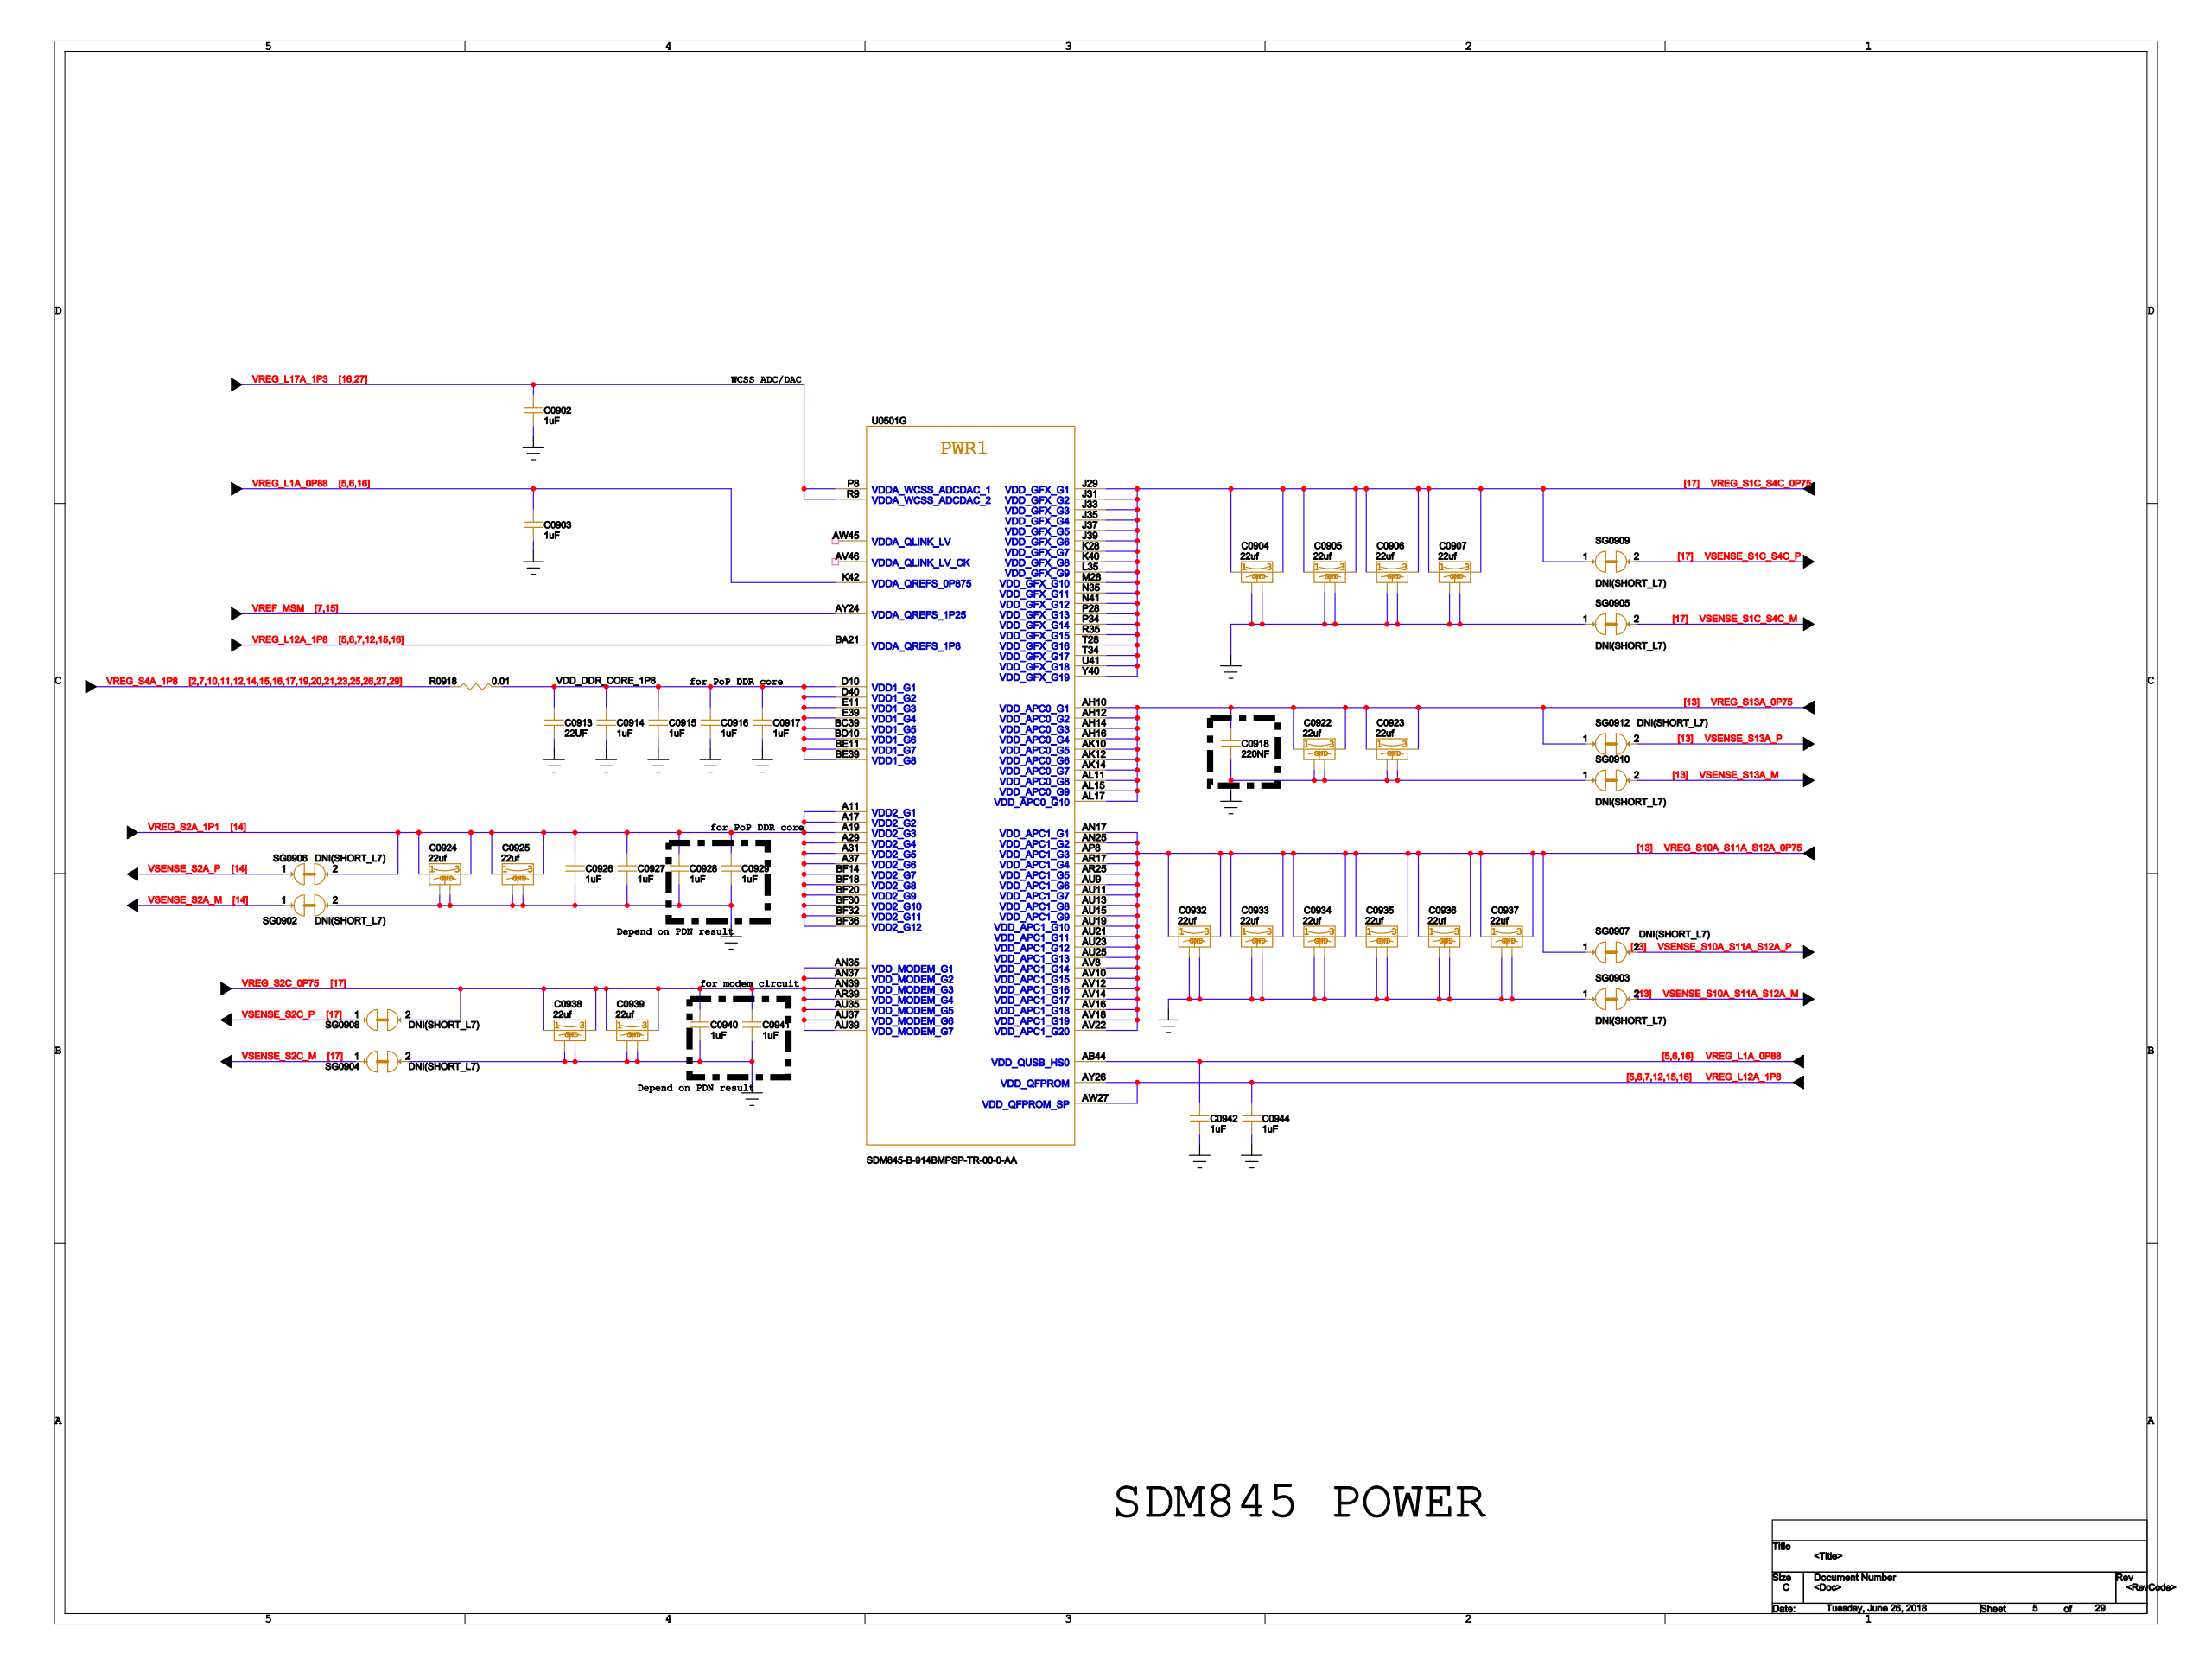Circuit board | Cadence Allegro | 802 parts | 566 nets | one sheet of the schematic
Parts on this sheet (reference | value | footprint):
C0902 | 1uF | C0201
C0903 | 1uF | C0201
C0904 | 22uf | NFMJMPC226R0G3
C0905 | 22uf | NFMJMPC226R0G3
C0906 | 22uf | NFMJMPC226R0G3
C0907 | 22uf | NFMJMPC226R0G3
C0913 | 22UF | 0603-BIG
C0914 | 1uF | C0201
C0915 | 1uF | C0201
C0916 | 1uF | C0201
C0917 | 1uF | C0201
C0918 | 220NF | C0201
C0922 | 22uf | NFMJMPC226R0G3
C0923 | 22uf | NFMJMPC226R0G3
C0924 | 22uf | NFMJMPC226R0G3
C0925 | 22uf | NFMJMPC226R0G3
C0926 | 1uF | C0201
C0927 | 1uF | C0201
C0928 | 1uF | C0201
C0929 | 1uF | C0201
C0932 | 22uf | NFMJMPC226R0G3
C0933 | 22uf | NFMJMPC226R0G3
C0934 | 22uf | NFMJMPC226R0G3
C0935 | 22uf | NFMJMPC226R0G3
C0936 | 22uf | NFMJMPC226R0G3
C0937 | 22uf | NFMJMPC226R0G3
C0938 | 22uf | NFMJMPC226R0G3
C0939 | 22uf | NFMJMPC226R0G3
C0940 | 1uF | C0201
C0941 | 1uF | C0201
C0942 | 1uF | C0201
C0944 | 1uF | C0201
R0918 | 0.01 | R0603
SG0902 | DNI(SHORT_L7) | SHORT_L7_2REC08X12
SG0903 | DNI(SHORT_L7) | SHORT_L7_2REC08X12
SG0904 | DNI(SHORT_L7) | SHORT_L7_2REC08X12
SG0905 | DNI(SHORT_L7) | SHORT_L7_2REC08X12
SG0906 | DNI(SHORT_L7) | SHORT_L7_2REC08X12
SG0907 | DNI(SHORT_L7) | SHORT_L7_2REC08X12
SG0908 | DNI(SHORT_L7) | SHORT_L7_2REC08X12
SG0909 | DNI(SHORT_L7) | SHORT_L7_2REC08X12
SG0910 | DNI(SHORT_L7) | SHORT_L7_2REC08X12
SG0912 | DNI(SHORT_L7) | SHORT_L7_2REC08X12
U0501 | SDM845-B-914BMPSP-TR-00-0-AA | BGA914_12P4X12P4_0P58_0P35
Nets of these parts (net: part-pin ...):
GND: C0902-2 C0903-2 C0904-2 C0904-4 C0905-2 C0905-4 C0906-2 C0906-4 C0907-2 C0907-4 C0913-2 C0914-2 C0915-2 C0916-2 C0917-2 C0918-2 C0922-2 C0922-4 C0923-2 C0923-4 C0924-2 C0924-4 C0925-2 C0925-4 C0926-2 C0927-2 C0928-2 C0929-2 C0932-2 C0932-4 C0933-2 C0933-4 C0934-2 C0934-4 C0935-2 C0935-4 C0936-2 C0936-4 C0937-2 C0937-4 C0938-2 C0938-4 C0939-2 C0939-4 C0940-2 C0941-2 C0942-2 C0944-2 SG0902-2 SG0903-1 SG0904-2 SG0905-1 SG0910-1
VREF_MSM: U0501-AY24
VREG_S4A_1P8: R0918-1
VREG_L17A_1P3: C0902-1 U0501-P8 U0501-R9
VREG_L1A_0P88: C0903-1 C0942-1 U0501-AB44 U0501-K42
VDD_DDR_CORE_1P8: C0913-1 C0914-1 C0915-1 C0916-1 C0917-1 R0918-2 U0501-BC39 U0501-BD10 U0501-BE11 U0501-BE39 U0501-D10 U0501-D40 U0501-E11 U0501-E39
VREG_S2A_1P1: C0924-1 C0924-3 C0925-1 C0925-3 C0926-1 C0927-1 C0928-1 C0929-1 SG0906-2 U0501-A11 U0501-A17 U0501-A19 U0501-A29 U0501-A31 U0501-A37 U0501-BF14 U0501-BF18 U0501-BF20 U0501-BF30 U0501-BF32 U0501-BF36
VREG_S2C_0P75: C0938-1 C0938-3 C0939-1 C0939-3 C0940-1 C0941-1 SG0908-2 U0501-AN35 U0501-AN37 U0501-AN39 U0501-AR39 U0501-AU35 U0501-AU37 U0501-AU39
VREG_L12A_1P8: C0944-1 U0501-AW27 U0501-AY26 U0501-BA21
VREG_S13A_0P75: C0918-1 C0922-1 C0922-3 C0923-1 C0923-3 SG0912-1 U0501-AH10 U0501-AH12 U0501-AH14 U0501-AH16 U0501-AK10 U0501-AK12 U0501-AK14 U0501-AL11 U0501-AL15 U0501-AL17
VREG_S1C_S4C_0P75: C0904-1 C0904-3 C0905-1 C0905-3 C0906-1 C0906-3 C0907-1 C0907-3 SG0909-1 U0501-J29 U0501-J31 U0501-J33 U0501-J35 U0501-J37 U0501-J39 U0501-K28 U0501-K40 U0501-L35 U0501-M28 U0501-N35 U0501-N41 U0501-P28 U0501-P34 U0501-R35 U0501-T28 U0501-T34 U0501-U41 U0501-Y40
VREG_S10A_S11A_S12A_0P75: C0932-1 C0932-3 C0933-1 C0933-3 C0934-1 C0934-3 C0935-1 C0935-3 C0936-1 C0936-3 C0937-1 C0937-3 SG0907-1 U0501-AN17 U0501-AN25 U0501-AP8 U0501-AR17 U0501-AR25 U0501-AU9 U0501-AU11 U0501-AU13 U0501-AU15 U0501-AU19 U0501-AU21 U0501-AU23 U0501-AU25 U0501-AV8 U0501-AV10 U0501-AV12 U0501-AV14 U0501-AV16 U0501-AV18 U0501-AV22
VSENSE_S2A_M: SG0902-1
VSENSE_S10A_S11A_S12A_M: SG0903-2
VSENSE_S2C_M: SG0904-1
VSENSE_S1C_S4C_M: SG0905-2
VSENSE_S2A_P: SG0906-1
VSENSE_S10A_S11A_S12A_P: SG0907-2
VSENSE_S2C_P: SG0908-1
VSENSE_S1C_S4C_P: SG0909-2
VSENSE_S13A_M: SG0910-2
VSENSE_S13A_P: SG0912-2